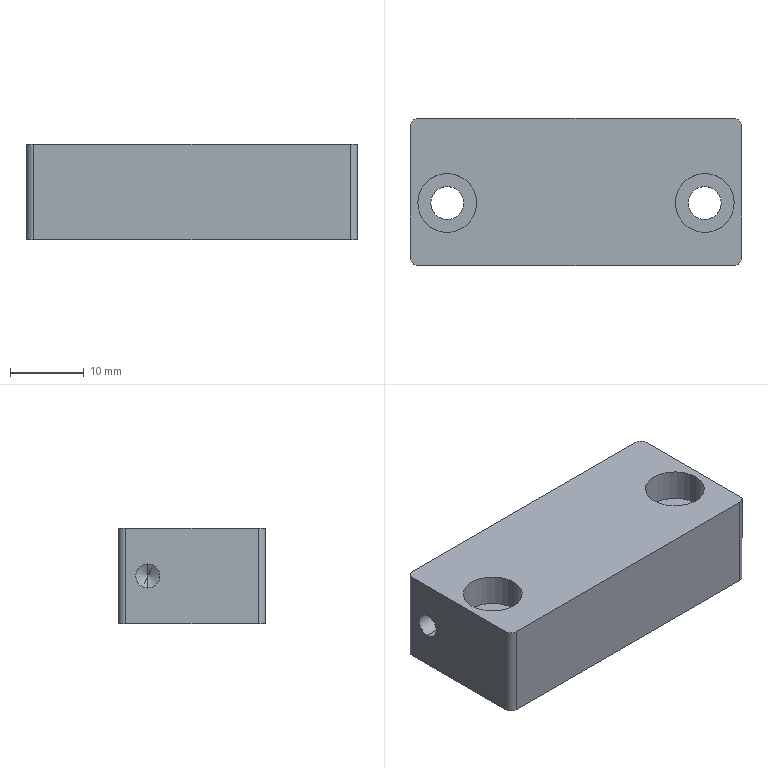Part | STEP file | 1 solid | 28 faces | box 45 x 20 x 13 mm | volume 10795 mm3 | cylinder 16 | plane 8 | cone 4 | commonest cylinder face diameters 2 x4 3.3 x4 4.5 x4 8 x4